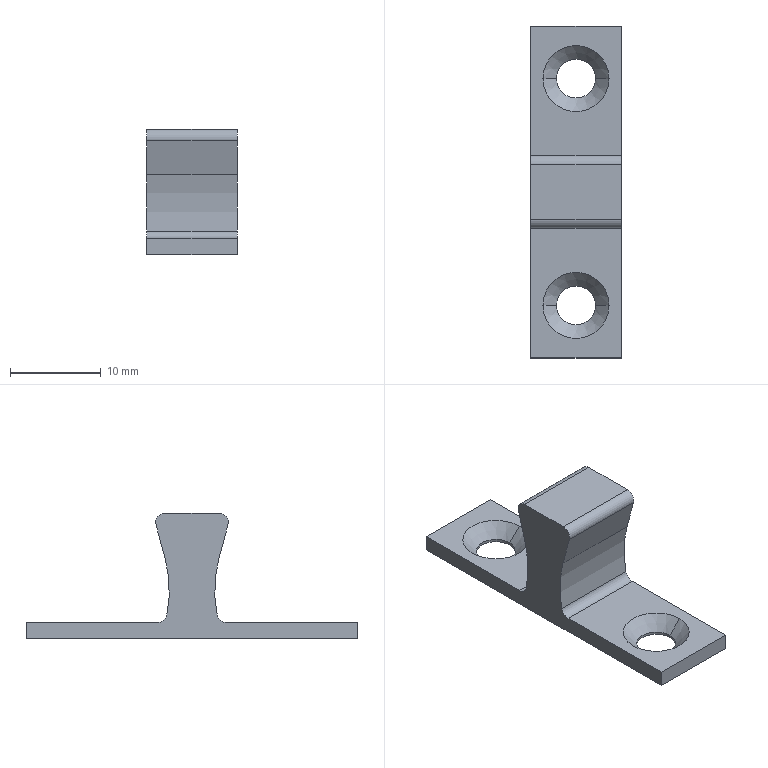Part | STEP file | door stop B | 1 solid | 24 faces | box 10 x 36.6 x 13.8 mm | volume 1298 mm3 | cylinder 10 | plane 10 | cone 4 | commonest cylinder face diameters 2 x4 4.3 x4 26.999 x2